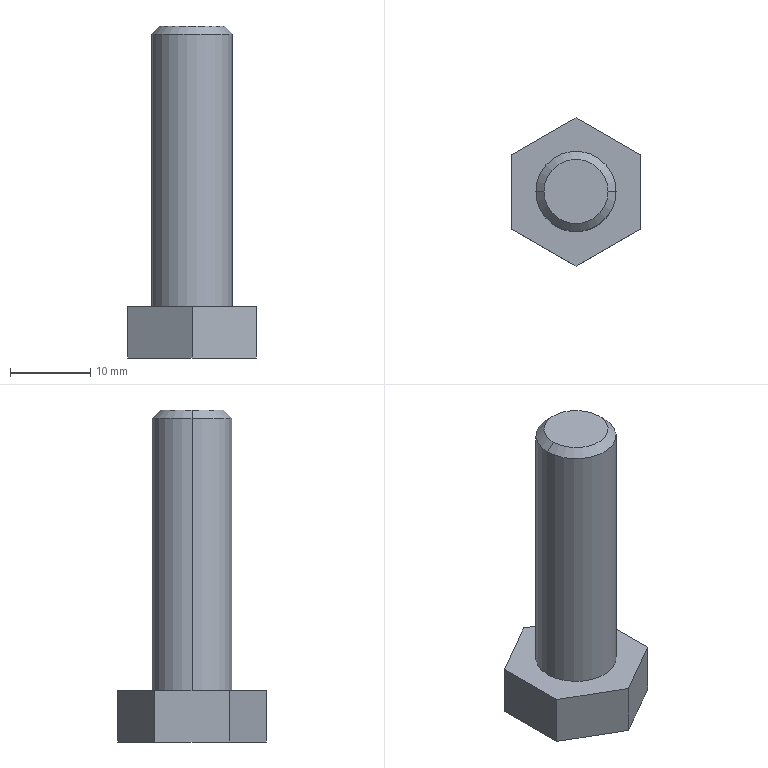Part | SolidWorks | features Chamfer 1, Extrusion 1, ICE 1, RefAxis 1 | 1 solid | 13 faces | box 16 x 18.475 x 41.4 mm | volume 4153 mm3 | plane 9 | cone 2 | cylinder 2 | commonest cylinder face diameters 10 x2
STEP:
#1=CARTESIAN_POINT('',(4.,0.,41.4));
#2=VERTEX_POINT('',#1);
#3=CARTESIAN_POINT('',(-4.,0.,41.4));
#4=VERTEX_POINT('',#3);
#5=CARTESIAN_POINT('',(0.,0.,41.4));
#6=DIRECTION('',(0.,0.,1.));
#7=DIRECTION('',(1.,0.,0.));
#8=AXIS2_PLACEMENT_3D('',#5,#6,#7);
#9=CIRCLE('',#8,4.);
#10=EDGE_CURVE('',#2,#4,#9,.T.);
#11=ORIENTED_EDGE('',*,*,#10,.F.);
#12=CARTESIAN_POINT('',(5.,0.,40.4));
#13=VERTEX_POINT('',#12);
#14=CARTESIAN_POINT('',(4.,0.,41.4));
#15=DIRECTION('',(0.7071,0.,-0.7071));
#16=VECTOR('',#15,1000.);
#17=LINE('',#14,#16);
#18=EDGE_CURVE('',#2,#13,#17,.T.);
#19=ORIENTED_EDGE('',*,*,#18,.T.);
#20=CARTESIAN_POINT('',(-5.,0.,40.4));
#21=VERTEX_POINT('',#20);
#22=CARTESIAN_POINT('',(0.,0.,40.4));
#23=DIRECTION('',(0.,0.,-1.));
#24=DIRECTION('',(1.,0.,0.));
#25=AXIS2_PLACEMENT_3D('',#22,#23,#24);
#26=CIRCLE('',#25,5.);
#27=EDGE_CURVE('',#21,#13,#26,.T.);
#28=ORIENTED_EDGE('',*,*,#27,.F.);
#29=CARTESIAN_POINT('',(-4.,0.,41.4));
#30=DIRECTION('',(-0.7071,0.,-0.7071));
#31=VECTOR('',#30,1000.);
#32=LINE('',#29,#31);
#33=EDGE_CURVE('',#4,#21,#32,.T.);
#34=ORIENTED_EDGE('',*,*,#33,.F.);
#35=EDGE_LOOP('',(#11,#19,#28,#34));
#36=FACE_OUTER_BOUND('',#35,.T.);
#37=CARTESIAN_POINT('',(0.,0.,41.4));
#38=DIRECTION('',(0.,0.,-1.));
#39=DIRECTION('',(-1.,0.,0.));
#40=AXIS2_PLACEMENT_3D('',#37,#38,#39);
#41=CONICAL_SURFACE('',#40,4.,0.7854);
#42=ADVANCED_FACE('',(#36),#41,.T.);
#43=ORIENTED_EDGE('',*,*,#27,.T.);
#44=CARTESIAN_POINT('',(5.,0.,6.4));
#45=VERTEX_POINT('',#44);
#46=CARTESIAN_POINT('',(5.,0.,41.4));
#47=DIRECTION('',(0.,0.,-1.));
#48=VECTOR('',#47,1000.);
#49=LINE('',#46,#48);
#50=EDGE_CURVE('',#13,#45,#49,.T.);
#51=ORIENTED_EDGE('',*,*,#50,.T.);
#52=CARTESIAN_POINT('',(-5.,0.,6.4));
#53=VERTEX_POINT('',#52);
#54=CARTESIAN_POINT('',(0.,0.,6.4));
#55=DIRECTION('',(0.,0.,1.));
#56=DIRECTION('',(1.,0.,0.));
#57=AXIS2_PLACEMENT_3D('',#54,#55,#56);
#58=CIRCLE('',#57,5.);
#59=EDGE_CURVE('',#45,#53,#58,.T.);
#60=ORIENTED_EDGE('',*,*,#59,.T.);
#61=CARTESIAN_POINT('',(-5.,0.,41.4));
#62=DIRECTION('',(0.,0.,-1.));
#63=VECTOR('',#62,1000.);
#64=LINE('',#61,#63);
#65=EDGE_CURVE('',#21,#53,#64,.T.);
#66=ORIENTED_EDGE('',*,*,#65,.F.);
#67=EDGE_LOOP('',(#43,#51,#60,#66));
#68=FACE_OUTER_BOUND('',#67,.T.);
#69=CARTESIAN_POINT('',(0.,0.,41.4));
#70=DIRECTION('',(0.,0.,-1.));
#71=DIRECTION('',(-1.,0.,0.));
#72=AXIS2_PLACEMENT_3D('',#69,#70,#71);
#73=CYLINDRICAL_SURFACE('',#72,5.);
#74=ADVANCED_FACE('',(#68),#73,.T.);
#75=CARTESIAN_POINT('',(8.,-4.619,6.4));
#76=VERTEX_POINT('',#75);
#77=CARTESIAN_POINT('',(8.,4.619,6.4));
#78=VERTEX_POINT('',#77);
#79=CARTESIAN_POINT('',(8.,-4.619,6.4));
#80=DIRECTION('',(0.,1.,0.));
#81=VECTOR('',#80,1000.);
#82=LINE('',#79,#81);
#83=EDGE_CURVE('',#76,#78,#82,.T.);
#84=ORIENTED_EDGE('',*,*,#83,.T.);
#85=CARTESIAN_POINT('',(0.,9.238,6.4));
#86=VERTEX_POINT('',#85);
#87=CARTESIAN_POINT('',(8.,4.619,6.4));
#88=DIRECTION('',(-0.866,0.5,0.));
#89=VECTOR('',#88,1000.);
#90=LINE('',#87,#89);
#91=EDGE_CURVE('',#78,#86,#90,.T.);
#92=ORIENTED_EDGE('',*,*,#91,.T.);
#93=CARTESIAN_POINT('',(-8.,4.619,6.4));
#94=VERTEX_POINT('',#93);
#95=CARTESIAN_POINT('',(0.,9.238,6.4));
#96=DIRECTION('',(-0.866,-0.5,0.));
#97=VECTOR('',#96,1000.);
#98=LINE('',#95,#97);
#99=EDGE_CURVE('',#86,#94,#98,.T.);
#100=ORIENTED_EDGE('',*,*,#99,.T.);
#101=CARTESIAN_POINT('',(-8.,-4.619,6.4));
#102=VERTEX_POINT('',#101);
#103=CARTESIAN_POINT('',(-8.,4.619,6.4));
#104=DIRECTION('',(0.,-1.,0.));
#105=VECTOR('',#104,1000.);
#106=LINE('',#103,#105);
#107=EDGE_CURVE('',#94,#102,#106,.T.);
#108=ORIENTED_EDGE('',*,*,#107,.T.);
#109=CARTESIAN_POINT('',(0.,-9.238,6.4));
#110=VERTEX_POINT('',#109);
#111=CARTESIAN_POINT('',(-8.,-4.619,6.4));
#112=DIRECTION('',(0.866,-0.5,0.));
#113=VECTOR('',#112,1000.);
#114=LINE('',#111,#113);
#115=EDGE_CURVE('',#102,#110,#114,.T.);
#116=ORIENTED_EDGE('',*,*,#115,.T.);
#117=CARTESIAN_POINT('',(0.,-9.238,6.4));
#118=DIRECTION('',(0.866,0.5,0.));
#119=VECTOR('',#118,1000.);
#120=LINE('',#117,#119);
#121=EDGE_CURVE('',#110,#76,#120,.T.);
#122=ORIENTED_EDGE('',*,*,#121,.T.);
#123=EDGE_LOOP('',(#84,#92,#100,#108,#116,#122));
#124=FACE_OUTER_BOUND('',#123,.T.);
#125=CARTESIAN_POINT('',(0.,0.,6.4));
#126=DIRECTION('',(0.,0.,1.));
#127=DIRECTION('',(1.,0.,0.));
#128=AXIS2_PLACEMENT_3D('',#125,#126,#127);
#129=CIRCLE('',#128,5.);
#130=EDGE_CURVE('',#53,#45,#129,.T.);
#131=ORIENTED_EDGE('',*,*,#130,.F.);
#132=ORIENTED_EDGE('',*,*,#59,.F.);
#133=EDGE_LOOP('',(#131,#132));
#134=FACE_BOUND('',#133,.T.);
#135=CARTESIAN_POINT('',(0.,0.,6.4));
#136=DIRECTION('',(0.,0.,1.));
#137=DIRECTION('',(1.,0.,0.));
#138=AXIS2_PLACEMENT_3D('',#135,#136,#137);
#139=PLANE('',#138);
#140=ADVANCED_FACE('',(#124,#134),#139,.T.);
#141=CARTESIAN_POINT('',(8.,-4.619,0.));
#142=VERTEX_POINT('',#141);
#143=CARTESIAN_POINT('',(8.,4.619,0.));
#144=VERTEX_POINT('',#143);
#145=CARTESIAN_POINT('',(8.,-4.619,0.));
#146=DIRECTION('',(0.,1.,0.));
#147=VECTOR('',#146,1000.);
#148=LINE('',#145,#147);
#149=EDGE_CURVE('',#142,#144,#148,.T.);
#150=ORIENTED_EDGE('',*,*,#149,.T.);
#151=CARTESIAN_POINT('',(8.,4.619,6.4));
#152=DIRECTION('',(0.,0.,-1.));
#153=VECTOR('',#152,1000.);
#154=LINE('',#151,#153);
#155=EDGE_CURVE('',#78,#144,#154,.T.);
#156=ORIENTED_EDGE('',*,*,#155,.F.);
#157=ORIENTED_EDGE('',*,*,#83,.F.);
#158=CARTESIAN_POINT('',(8.,-4.619,6.4));
#159=DIRECTION('',(0.,0.,-1.));
#160=VECTOR('',#159,1000.);
#161=LINE('',#158,#160);
#162=EDGE_CURVE('',#76,#142,#161,.T.);
#163=ORIENTED_EDGE('',*,*,#162,.T.);
#164=EDGE_LOOP('',(#150,#156,#157,#163));
#165=FACE_OUTER_BOUND('',#164,.T.);
#166=CARTESIAN_POINT('',(8.,-4.619,6.4));
#167=DIRECTION('',(-1.,0.,0.));
#168=DIRECTION('',(0.,-1.,0.));
#169=AXIS2_PLACEMENT_3D('',#166,#167,#168);
#170=PLANE('',#169);
#171=ADVANCED_FACE('',(#165),#170,.F.);
#172=CARTESIAN_POINT('',(0.,9.238,0.));
#173=VERTEX_POINT('',#172);
#174=CARTESIAN_POINT('',(8.,4.619,0.));
#175=DIRECTION('',(-0.866,0.5,0.));
#176=VECTOR('',#175,1000.);
#177=LINE('',#174,#176);
#178=EDGE_CURVE('',#144,#173,#177,.T.);
#179=ORIENTED_EDGE('',*,*,#178,.T.);
#180=CARTESIAN_POINT('',(0.,9.238,6.4));
#181=DIRECTION('',(0.,0.,-1.));
#182=VECTOR('',#181,1000.);
#183=LINE('',#180,#182);
#184=EDGE_CURVE('',#86,#173,#183,.T.);
#185=ORIENTED_EDGE('',*,*,#184,.F.);
#186=ORIENTED_EDGE('',*,*,#91,.F.);
#187=ORIENTED_EDGE('',*,*,#155,.T.);
#188=EDGE_LOOP('',(#179,#185,#186,#187));
#189=FACE_OUTER_BOUND('',#188,.T.);
#190=CARTESIAN_POINT('',(8.,4.619,6.4));
#191=DIRECTION('',(-0.5,-0.866,0.));
#192=DIRECTION('',(0.866,-0.5,0.));
#193=AXIS2_PLACEMENT_3D('',#190,#191,#192);
#194=PLANE('',#193);
#195=ADVANCED_FACE('',(#189),#194,.F.);
#196=CARTESIAN_POINT('',(-8.,4.619,0.));
#197=VERTEX_POINT('',#196);
#198=CARTESIAN_POINT('',(0.,9.238,0.));
#199=DIRECTION('',(-0.866,-0.5,0.));
#200=VECTOR('',#199,1000.);
#201=LINE('',#198,#200);
#202=EDGE_CURVE('',#173,#197,#201,.T.);
#203=ORIENTED_EDGE('',*,*,#202,.T.);
#204=CARTESIAN_POINT('',(-8.,4.619,6.4));
#205=DIRECTION('',(0.,0.,-1.));
#206=VECTOR('',#205,1000.);
#207=LINE('',#204,#206);
#208=EDGE_CURVE('',#94,#197,#207,.T.);
#209=ORIENTED_EDGE('',*,*,#208,.F.);
#210=ORIENTED_EDGE('',*,*,#99,.F.);
#211=ORIENTED_EDGE('',*,*,#184,.T.);
#212=EDGE_LOOP('',(#203,#209,#210,#211));
#213=FACE_OUTER_BOUND('',#212,.T.);
#214=CARTESIAN_POINT('',(0.,9.238,6.4));
#215=DIRECTION('',(0.5,-0.866,0.));
#216=DIRECTION('',(0.866,0.5,0.));
#217=AXIS2_PLACEMENT_3D('',#214,#215,#216);
#218=PLANE('',#217);
#219=ADVANCED_FACE('',(#213),#218,.F.);
#220=CARTESIAN_POINT('',(-8.,-4.619,0.));
#221=VERTEX_POINT('',#220);
#222=CARTESIAN_POINT('',(-8.,4.619,0.));
#223=DIRECTION('',(0.,-1.,0.));
#224=VECTOR('',#223,1000.);
#225=LINE('',#222,#224);
#226=EDGE_CURVE('',#197,#221,#225,.T.);
#227=ORIENTED_EDGE('',*,*,#226,.T.);
#228=CARTESIAN_POINT('',(-8.,-4.619,6.4));
#229=DIRECTION('',(0.,0.,-1.));
#230=VECTOR('',#229,1000.);
#231=LINE('',#228,#230);
#232=EDGE_CURVE('',#102,#221,#231,.T.);
#233=ORIENTED_EDGE('',*,*,#232,.F.);
#234=ORIENTED_EDGE('',*,*,#107,.F.);
#235=ORIENTED_EDGE('',*,*,#208,.T.);
#236=EDGE_LOOP('',(#227,#233,#234,#235));
#237=FACE_OUTER_BOUND('',#236,.T.);
#238=CARTESIAN_POINT('',(-8.,4.619,6.4));
#239=DIRECTION('',(1.,0.,0.));
#240=DIRECTION('',(0.,1.,0.));
#241=AXIS2_PLACEMENT_3D('',#238,#239,#240);
#242=PLANE('',#241);
#243=ADVANCED_FACE('',(#237),#242,.F.);
#244=CARTESIAN_POINT('',(0.,-9.238,0.));
#245=VERTEX_POINT('',#244);
#246=CARTESIAN_POINT('',(-8.,-4.619,0.));
#247=DIRECTION('',(0.866,-0.5,0.));
#248=VECTOR('',#247,1000.);
#249=LINE('',#246,#248);
#250=EDGE_CURVE('',#221,#245,#249,.T.);
#251=ORIENTED_EDGE('',*,*,#250,.T.);
#252=CARTESIAN_POINT('',(0.,-9.238,6.4));
#253=DIRECTION('',(0.,0.,-1.));
#254=VECTOR('',#253,1000.);
#255=LINE('',#252,#254);
#256=EDGE_CURVE('',#110,#245,#255,.T.);
#257=ORIENTED_EDGE('',*,*,#256,.F.);
#258=ORIENTED_EDGE('',*,*,#115,.F.);
#259=ORIENTED_EDGE('',*,*,#232,.T.);
#260=EDGE_LOOP('',(#251,#257,#258,#259));
#261=FACE_OUTER_BOUND('',#260,.T.);
#262=CARTESIAN_POINT('',(-8.,-4.619,6.4));
#263=DIRECTION('',(0.5,0.866,0.));
#264=DIRECTION('',(-0.866,0.5,0.));
#265=AXIS2_PLACEMENT_3D('',#262,#263,#264);
#266=PLANE('',#265);
#267=ADVANCED_FACE('',(#261),#266,.F.);
#268=CARTESIAN_POINT('',(0.,-9.238,0.));
#269=DIRECTION('',(0.866,0.5,0.));
#270=VECTOR('',#269,1000.);
#271=LINE('',#268,#270);
#272=EDGE_CURVE('',#245,#142,#271,.T.);
#273=ORIENTED_EDGE('',*,*,#272,.T.);
#274=ORIENTED_EDGE('',*,*,#162,.F.);
#275=ORIENTED_EDGE('',*,*,#121,.F.);
#276=ORIENTED_EDGE('',*,*,#256,.T.);
#277=EDGE_LOOP('',(#273,#274,#275,#276));
#278=FACE_OUTER_BOUND('',#277,.T.);
#279=CARTESIAN_POINT('',(0.,-9.238,6.4));
#280=DIRECTION('',(-0.5,0.866,0.));
#281=DIRECTION('',(-0.866,-0.5,0.));
#282=AXIS2_PLACEMENT_3D('',#279,#280,#281);
#283=PLANE('',#282);
#284=ADVANCED_FACE('',(#278),#283,.F.);
#285=ORIENTED_EDGE('',*,*,#149,.F.);
#286=ORIENTED_EDGE('',*,*,#272,.F.);
#287=ORIENTED_EDGE('',*,*,#250,.F.);
#288=ORIENTED_EDGE('',*,*,#226,.F.);
#289=ORIENTED_EDGE('',*,*,#202,.F.);
#290=ORIENTED_EDGE('',*,*,#178,.F.);
#291=EDGE_LOOP('',(#285,#286,#287,#288,#289,#290));
#292=FACE_OUTER_BOUND('',#291,.T.);
#293=CARTESIAN_POINT('',(0.,0.,0.));
#294=DIRECTION('',(0.,0.,1.));
#295=DIRECTION('',(1.,0.,0.));
#296=AXIS2_PLACEMENT_3D('',#293,#294,#295);
#297=PLANE('',#296);
#298=ADVANCED_FACE('',(#292),#297,.F.);
#299=ORIENTED_EDGE('',*,*,#50,.F.);
#300=CARTESIAN_POINT('',(0.,0.,40.4));
#301=DIRECTION('',(0.,0.,-1.));
#302=DIRECTION('',(1.,0.,0.));
#303=AXIS2_PLACEMENT_3D('',#300,#301,#302);
#304=CIRCLE('',#303,5.);
#305=EDGE_CURVE('',#13,#21,#304,.T.);
#306=ORIENTED_EDGE('',*,*,#305,.T.);
#307=ORIENTED_EDGE('',*,*,#65,.T.);
#308=ORIENTED_EDGE('',*,*,#130,.T.);
#309=EDGE_LOOP('',(#299,#306,#307,#308));
#310=FACE_OUTER_BOUND('',#309,.T.);
#311=CARTESIAN_POINT('',(0.,0.,41.4));
#312=DIRECTION('',(0.,0.,-1.));
#313=DIRECTION('',(-1.,0.,0.));
#314=AXIS2_PLACEMENT_3D('',#311,#312,#313);
#315=CYLINDRICAL_SURFACE('',#314,5.);
#316=ADVANCED_FACE('',(#310),#315,.T.);
#317=CARTESIAN_POINT('',(0.,0.,41.4));
#318=DIRECTION('',(0.,0.,1.));
#319=DIRECTION('',(1.,0.,0.));
#320=AXIS2_PLACEMENT_3D('',#317,#318,#319);
#321=CIRCLE('',#320,4.);
#322=EDGE_CURVE('',#4,#2,#321,.T.);
#323=ORIENTED_EDGE('',*,*,#322,.T.);
#324=ORIENTED_EDGE('',*,*,#10,.T.);
#325=EDGE_LOOP('',(#323,#324));
#326=FACE_OUTER_BOUND('',#325,.T.);
#327=CARTESIAN_POINT('',(0.,0.,41.4));
#328=DIRECTION('',(0.,0.,1.));
#329=DIRECTION('',(1.,0.,0.));
#330=AXIS2_PLACEMENT_3D('',#327,#328,#329);
#331=PLANE('',#330);
#332=ADVANCED_FACE('',(#326),#331,.T.);
#333=ORIENTED_EDGE('',*,*,#18,.F.);
#334=ORIENTED_EDGE('',*,*,#322,.F.);
#335=ORIENTED_EDGE('',*,*,#33,.T.);
#336=ORIENTED_EDGE('',*,*,#305,.F.);
#337=EDGE_LOOP('',(#333,#334,#335,#336));
#338=FACE_OUTER_BOUND('',#337,.T.);
#339=CARTESIAN_POINT('',(0.,0.,41.4));
#340=DIRECTION('',(0.,0.,-1.));
#341=DIRECTION('',(-1.,0.,0.));
#342=AXIS2_PLACEMENT_3D('',#339,#340,#341);
#343=CONICAL_SURFACE('',#342,4.,0.7854);
#344=ADVANCED_FACE('',(#338),#343,.T.);
#345=CLOSED_SHELL('',(#42,#74,#140,#171,#195,#219,#243,#267,#284,#298,#316,#332,#344));
#346=MANIFOLD_SOLID_BREP('',#345);
#347=CARTESIAN_POINT('',(0.,0.,0.));
#348=DIRECTION('',(0.,0.,1.));
#349=DIRECTION('',(1.,0.,0.));
#350=AXIS2_PLACEMENT_3D('',#347,#348,#349);
#351=(LENGTH_UNIT()NAMED_UNIT(*)SI_UNIT(.MILLI.,.METRE.));
#352=UNCERTAINTY_MEASURE_WITH_UNIT(LENGTH_MEASURE(0.00001),#351,'','');
#353=(NAMED_UNIT(*)PLANE_ANGLE_UNIT()SI_UNIT($,.RADIAN.));
#354=(NAMED_UNIT(*)SI_UNIT($,.STERADIAN.)SOLID_ANGLE_UNIT());
#355=(GEOMETRIC_REPRESENTATION_CONTEXT(3)GLOBAL_UNCERTAINTY_ASSIGNED_CONTEXT((#352))GLOBAL_UNIT_ASSIGNED_CONTEXT((#351,#353,#354))REPRESENTATION_CONTEXT('',''));
#356=ADVANCED_BREP_SHAPE_REPRESENTATION('',(#346,#350),#355);